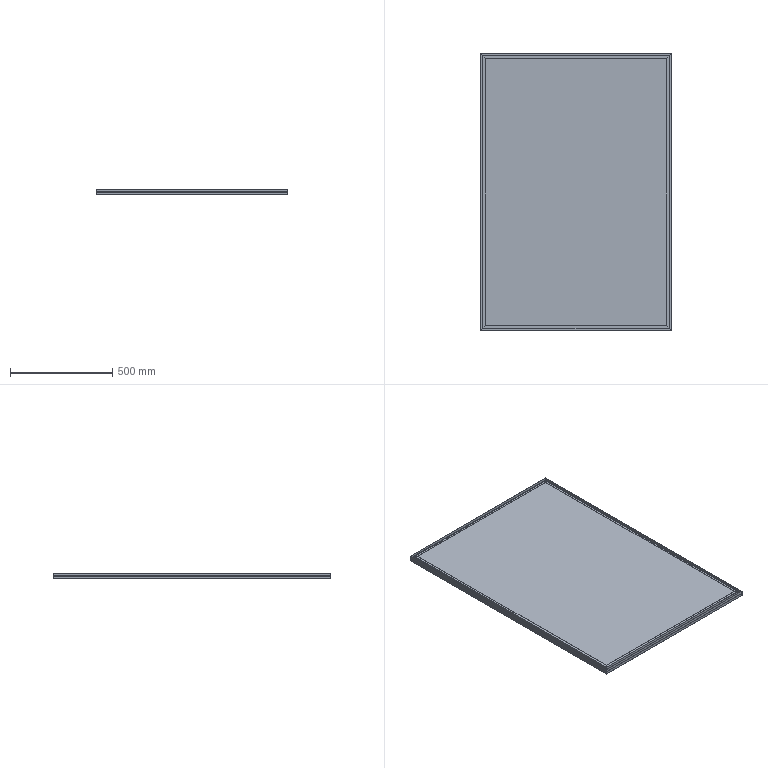Part | SolidWorks | features ICE 1, WeldMemberFeat 1, WeldmentFeature 1 | 5 solids | 78 faces | box 940 x 1360 x 27 mm | volume 27359520 mm3 | plane 78